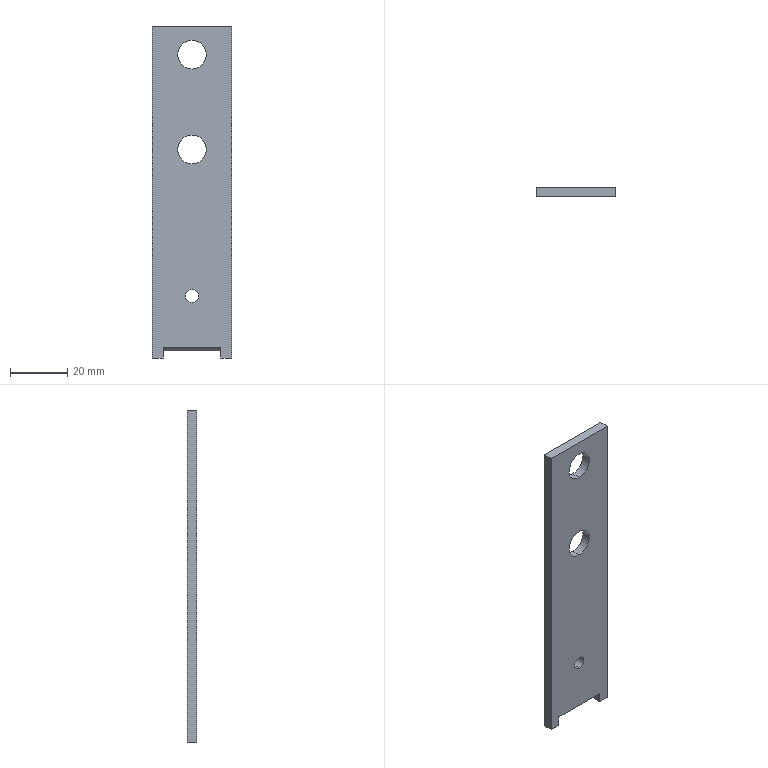Part | SolidWorks | features Chamfer 1, FlatPattern 1, SMBaseFlange 1, SheetMetal 1 | 1 solid | 18 faces | box 27.6 x 3.2 x 115.6 mm | volume 9476 mm3 | plane 12 | cylinder 6 | commonest cylinder face diameters 10 x4 4.5 x2
STEP:
#1=CARTESIAN_POINT('',(13.8,-3.2,-96.25));
#2=VERTEX_POINT('',#1);
#3=CARTESIAN_POINT('',(13.8,-3.2,-91.75));
#4=VERTEX_POINT('',#3);
#5=CARTESIAN_POINT('',(13.8,-3.2,-94.));
#6=DIRECTION('',(0.,1.,0.));
#7=DIRECTION('',(0.,0.,1.));
#8=AXIS2_PLACEMENT_3D('',#5,#6,#7);
#9=CIRCLE('',#8,2.25);
#10=EDGE_CURVE('',#2,#4,#9,.T.);
#11=ORIENTED_EDGE('',*,*,#10,.F.);
#12=CARTESIAN_POINT('',(13.8,0.,-96.25));
#13=VERTEX_POINT('',#12);
#14=CARTESIAN_POINT('',(13.8,-3.2,-96.25));
#15=DIRECTION('',(0.,1.,0.));
#16=VECTOR('',#15,1000.);
#17=LINE('',#14,#16);
#18=EDGE_CURVE('',#2,#13,#17,.T.);
#19=ORIENTED_EDGE('',*,*,#18,.T.);
#20=CARTESIAN_POINT('',(13.8,0.,-91.75));
#21=VERTEX_POINT('',#20);
#22=CARTESIAN_POINT('',(13.8,0.,-94.));
#23=DIRECTION('',(0.,1.,0.));
#24=DIRECTION('',(0.,0.,1.));
#25=AXIS2_PLACEMENT_3D('',#22,#23,#24);
#26=CIRCLE('',#25,2.25);
#27=EDGE_CURVE('',#13,#21,#26,.T.);
#28=ORIENTED_EDGE('',*,*,#27,.T.);
#29=CARTESIAN_POINT('',(13.8,-3.2,-91.75));
#30=DIRECTION('',(0.,1.,0.));
#31=VECTOR('',#30,1000.);
#32=LINE('',#29,#31);
#33=EDGE_CURVE('',#4,#21,#32,.T.);
#34=ORIENTED_EDGE('',*,*,#33,.F.);
#35=EDGE_LOOP('',(#11,#19,#28,#34));
#36=FACE_OUTER_BOUND('',#35,.T.);
#37=CARTESIAN_POINT('',(13.8,-3.2,-94.));
#38=DIRECTION('',(0.,1.,0.));
#39=DIRECTION('',(0.,0.,1.));
#40=AXIS2_PLACEMENT_3D('',#37,#38,#39);
#41=CYLINDRICAL_SURFACE('',#40,2.25);
#42=ADVANCED_FACE('',(#36),#41,.F.);
#43=CARTESIAN_POINT('',(13.8,-3.2,-48.));
#44=VERTEX_POINT('',#43);
#45=CARTESIAN_POINT('',(13.8,-3.2,-38.));
#46=VERTEX_POINT('',#45);
#47=CARTESIAN_POINT('',(13.8,-3.2,-43.));
#48=DIRECTION('',(0.,1.,0.));
#49=DIRECTION('',(0.,0.,1.));
#50=AXIS2_PLACEMENT_3D('',#47,#48,#49);
#51=CIRCLE('',#50,5.);
#52=EDGE_CURVE('',#44,#46,#51,.T.);
#53=ORIENTED_EDGE('',*,*,#52,.F.);
#54=CARTESIAN_POINT('',(13.8,0.,-48.));
#55=VERTEX_POINT('',#54);
#56=CARTESIAN_POINT('',(13.8,-3.2,-48.));
#57=DIRECTION('',(0.,1.,0.));
#58=VECTOR('',#57,1000.);
#59=LINE('',#56,#58);
#60=EDGE_CURVE('',#44,#55,#59,.T.);
#61=ORIENTED_EDGE('',*,*,#60,.T.);
#62=CARTESIAN_POINT('',(13.8,0.,-38.));
#63=VERTEX_POINT('',#62);
#64=CARTESIAN_POINT('',(13.8,0.,-43.));
#65=DIRECTION('',(0.,1.,0.));
#66=DIRECTION('',(0.,0.,1.));
#67=AXIS2_PLACEMENT_3D('',#64,#65,#66);
#68=CIRCLE('',#67,5.);
#69=EDGE_CURVE('',#55,#63,#68,.T.);
#70=ORIENTED_EDGE('',*,*,#69,.T.);
#71=CARTESIAN_POINT('',(13.8,-3.2,-38.));
#72=DIRECTION('',(0.,1.,0.));
#73=VECTOR('',#72,1000.);
#74=LINE('',#71,#73);
#75=EDGE_CURVE('',#46,#63,#74,.T.);
#76=ORIENTED_EDGE('',*,*,#75,.F.);
#77=EDGE_LOOP('',(#53,#61,#70,#76));
#78=FACE_OUTER_BOUND('',#77,.T.);
#79=CARTESIAN_POINT('',(13.8,-3.2,-43.));
#80=DIRECTION('',(0.,1.,0.));
#81=DIRECTION('',(0.,0.,1.));
#82=AXIS2_PLACEMENT_3D('',#79,#80,#81);
#83=CYLINDRICAL_SURFACE('',#82,5.);
#84=ADVANCED_FACE('',(#78),#83,.F.);
#85=CARTESIAN_POINT('',(13.8,-3.2,-15.));
#86=VERTEX_POINT('',#85);
#87=CARTESIAN_POINT('',(13.8,-3.2,-5.));
#88=VERTEX_POINT('',#87);
#89=CARTESIAN_POINT('',(13.8,-3.2,-10.));
#90=DIRECTION('',(0.,1.,0.));
#91=DIRECTION('',(0.,0.,1.));
#92=AXIS2_PLACEMENT_3D('',#89,#90,#91);
#93=CIRCLE('',#92,5.);
#94=EDGE_CURVE('',#86,#88,#93,.T.);
#95=ORIENTED_EDGE('',*,*,#94,.F.);
#96=CARTESIAN_POINT('',(13.8,0.,-15.));
#97=VERTEX_POINT('',#96);
#98=CARTESIAN_POINT('',(13.8,-3.2,-15.));
#99=DIRECTION('',(0.,1.,0.));
#100=VECTOR('',#99,1000.);
#101=LINE('',#98,#100);
#102=EDGE_CURVE('',#86,#97,#101,.T.);
#103=ORIENTED_EDGE('',*,*,#102,.T.);
#104=CARTESIAN_POINT('',(13.8,0.,-5.));
#105=VERTEX_POINT('',#104);
#106=CARTESIAN_POINT('',(13.8,0.,-10.));
#107=DIRECTION('',(0.,1.,0.));
#108=DIRECTION('',(0.,0.,1.));
#109=AXIS2_PLACEMENT_3D('',#106,#107,#108);
#110=CIRCLE('',#109,5.);
#111=EDGE_CURVE('',#97,#105,#110,.T.);
#112=ORIENTED_EDGE('',*,*,#111,.T.);
#113=CARTESIAN_POINT('',(13.8,-3.2,-5.));
#114=DIRECTION('',(0.,1.,0.));
#115=VECTOR('',#114,1000.);
#116=LINE('',#113,#115);
#117=EDGE_CURVE('',#88,#105,#116,.T.);
#118=ORIENTED_EDGE('',*,*,#117,.F.);
#119=EDGE_LOOP('',(#95,#103,#112,#118));
#120=FACE_OUTER_BOUND('',#119,.T.);
#121=CARTESIAN_POINT('',(13.8,-3.2,-10.));
#122=DIRECTION('',(0.,1.,0.));
#123=DIRECTION('',(0.,0.,1.));
#124=AXIS2_PLACEMENT_3D('',#121,#122,#123);
#125=CYLINDRICAL_SURFACE('',#124,5.);
#126=ADVANCED_FACE('',(#120),#125,.F.);
#127=CARTESIAN_POINT('',(0.,0.,-115.6));
#128=VERTEX_POINT('',#127);
#129=CARTESIAN_POINT('',(0.,0.,0.));
#130=VERTEX_POINT('',#129);
#131=CARTESIAN_POINT('',(0.,0.,0.));
#132=DIRECTION('',(0.,0.,1.));
#133=VECTOR('',#132,1000.);
#134=LINE('',#131,#133);
#135=EDGE_CURVE('',#128,#130,#134,.T.);
#136=ORIENTED_EDGE('',*,*,#135,.F.);
#137=CARTESIAN_POINT('',(0.,-3.2,-115.6));
#138=VERTEX_POINT('',#137);
#139=CARTESIAN_POINT('',(0.,-3.2,-115.6));
#140=DIRECTION('',(0.,1.,0.));
#141=VECTOR('',#140,1000.);
#142=LINE('',#139,#141);
#143=EDGE_CURVE('',#138,#128,#142,.T.);
#144=ORIENTED_EDGE('',*,*,#143,.F.);
#145=CARTESIAN_POINT('',(0.,-3.2,0.));
#146=VERTEX_POINT('',#145);
#147=CARTESIAN_POINT('',(0.,-3.2,0.));
#148=DIRECTION('',(0.,0.,1.));
#149=VECTOR('',#148,1000.);
#150=LINE('',#147,#149);
#151=EDGE_CURVE('',#138,#146,#150,.T.);
#152=ORIENTED_EDGE('',*,*,#151,.T.);
#153=CARTESIAN_POINT('',(0.,-3.2,0.));
#154=DIRECTION('',(0.,1.,0.));
#155=VECTOR('',#154,1000.);
#156=LINE('',#153,#155);
#157=EDGE_CURVE('',#146,#130,#156,.T.);
#158=ORIENTED_EDGE('',*,*,#157,.T.);
#159=EDGE_LOOP('',(#136,#144,#152,#158));
#160=FACE_OUTER_BOUND('',#159,.T.);
#161=CARTESIAN_POINT('',(0.,-3.2,0.));
#162=DIRECTION('',(-1.,0.,0.));
#163=DIRECTION('',(0.,0.,1.));
#164=AXIS2_PLACEMENT_3D('',#161,#162,#163);
#165=PLANE('',#164);
#166=ADVANCED_FACE('',(#160),#165,.T.);
#167=CARTESIAN_POINT('',(3.8,0.,-115.6));
#168=VERTEX_POINT('',#167);
#169=CARTESIAN_POINT('',(0.,0.,-115.6));
#170=DIRECTION('',(-1.,0.,0.));
#171=VECTOR('',#170,1000.);
#172=LINE('',#169,#171);
#173=EDGE_CURVE('',#168,#128,#172,.T.);
#174=ORIENTED_EDGE('',*,*,#173,.F.);
#175=CARTESIAN_POINT('',(3.8,-3.2,-115.6));
#176=VERTEX_POINT('',#175);
#177=CARTESIAN_POINT('',(3.8,-3.2,-115.6));
#178=DIRECTION('',(0.,1.,0.));
#179=VECTOR('',#178,1000.);
#180=LINE('',#177,#179);
#181=EDGE_CURVE('',#176,#168,#180,.T.);
#182=ORIENTED_EDGE('',*,*,#181,.F.);
#183=CARTESIAN_POINT('',(0.,-3.2,-115.6));
#184=DIRECTION('',(-1.,0.,0.));
#185=VECTOR('',#184,1000.);
#186=LINE('',#183,#185);
#187=EDGE_CURVE('',#176,#138,#186,.T.);
#188=ORIENTED_EDGE('',*,*,#187,.T.);
#189=ORIENTED_EDGE('',*,*,#143,.T.);
#190=EDGE_LOOP('',(#174,#182,#188,#189));
#191=FACE_OUTER_BOUND('',#190,.T.);
#192=CARTESIAN_POINT('',(0.,-3.2,-115.6));
#193=DIRECTION('',(0.,0.,-1.));
#194=DIRECTION('',(-1.,0.,0.));
#195=AXIS2_PLACEMENT_3D('',#192,#193,#194);
#196=PLANE('',#195);
#197=ADVANCED_FACE('',(#191),#196,.T.);
#198=CARTESIAN_POINT('',(3.8,0.,-112.1));
#199=VERTEX_POINT('',#198);
#200=CARTESIAN_POINT('',(3.8,0.,-115.6));
#201=DIRECTION('',(0.,0.,-1.));
#202=VECTOR('',#201,1000.);
#203=LINE('',#200,#202);
#204=EDGE_CURVE('',#199,#168,#203,.T.);
#205=ORIENTED_EDGE('',*,*,#204,.F.);
#206=CARTESIAN_POINT('',(3.8,-1.,-113.1));
#207=VERTEX_POINT('',#206);
#208=CARTESIAN_POINT('',(3.8,0.,-112.1));
#209=DIRECTION('',(0.,-0.7071,-0.7071));
#210=VECTOR('',#209,1000.);
#211=LINE('',#208,#210);
#212=EDGE_CURVE('',#199,#207,#211,.T.);
#213=ORIENTED_EDGE('',*,*,#212,.T.);
#214=CARTESIAN_POINT('',(3.8,-2.2,-113.1));
#215=VERTEX_POINT('',#214);
#216=CARTESIAN_POINT('',(3.8,-3.2,-113.1));
#217=DIRECTION('',(0.,1.,0.));
#218=VECTOR('',#217,1000.);
#219=LINE('',#216,#218);
#220=EDGE_CURVE('',#215,#207,#219,.T.);
#221=ORIENTED_EDGE('',*,*,#220,.F.);
#222=CARTESIAN_POINT('',(3.8,-3.2,-112.1));
#223=VERTEX_POINT('',#222);
#224=CARTESIAN_POINT('',(3.8,-2.2,-113.1));
#225=DIRECTION('',(0.,-0.7071,0.7071));
#226=VECTOR('',#225,1000.);
#227=LINE('',#224,#226);
#228=EDGE_CURVE('',#215,#223,#227,.T.);
#229=ORIENTED_EDGE('',*,*,#228,.T.);
#230=CARTESIAN_POINT('',(3.8,-3.2,-115.6));
#231=DIRECTION('',(0.,0.,-1.));
#232=VECTOR('',#231,1000.);
#233=LINE('',#230,#232);
#234=EDGE_CURVE('',#223,#176,#233,.T.);
#235=ORIENTED_EDGE('',*,*,#234,.T.);
#236=ORIENTED_EDGE('',*,*,#181,.T.);
#237=EDGE_LOOP('',(#205,#213,#221,#229,#235,#236));
#238=FACE_OUTER_BOUND('',#237,.T.);
#239=CARTESIAN_POINT('',(3.8,-3.2,-115.6));
#240=DIRECTION('',(1.,0.,0.));
#241=DIRECTION('',(0.,0.,-1.));
#242=AXIS2_PLACEMENT_3D('',#239,#240,#241);
#243=PLANE('',#242);
#244=ADVANCED_FACE('',(#238),#243,.T.);
#245=CARTESIAN_POINT('',(23.8,-2.2,-113.1));
#246=VERTEX_POINT('',#245);
#247=CARTESIAN_POINT('',(23.8,-1.,-113.1));
#248=VERTEX_POINT('',#247);
#249=CARTESIAN_POINT('',(23.8,-3.2,-113.1));
#250=DIRECTION('',(0.,1.,0.));
#251=VECTOR('',#250,1000.);
#252=LINE('',#249,#251);
#253=EDGE_CURVE('',#246,#248,#252,.T.);
#254=ORIENTED_EDGE('',*,*,#253,.F.);
#255=CARTESIAN_POINT('',(3.8,-2.2,-113.1));
#256=DIRECTION('',(-1.,0.,0.));
#257=VECTOR('',#256,1000.);
#258=LINE('',#255,#257);
#259=EDGE_CURVE('',#246,#215,#258,.T.);
#260=ORIENTED_EDGE('',*,*,#259,.T.);
#261=ORIENTED_EDGE('',*,*,#220,.T.);
#262=CARTESIAN_POINT('',(23.8,-1.,-113.1));
#263=DIRECTION('',(1.,0.,0.));
#264=VECTOR('',#263,1000.);
#265=LINE('',#262,#264);
#266=EDGE_CURVE('',#207,#248,#265,.T.);
#267=ORIENTED_EDGE('',*,*,#266,.T.);
#268=EDGE_LOOP('',(#254,#260,#261,#267));
#269=FACE_OUTER_BOUND('',#268,.T.);
#270=CARTESIAN_POINT('',(3.8,-3.2,-113.1));
#271=DIRECTION('',(0.,0.,-1.));
#272=DIRECTION('',(-1.,0.,0.));
#273=AXIS2_PLACEMENT_3D('',#270,#271,#272);
#274=PLANE('',#273);
#275=ADVANCED_FACE('',(#269),#274,.T.);
#276=CARTESIAN_POINT('',(23.8,0.,-115.6));
#277=VERTEX_POINT('',#276);
#278=CARTESIAN_POINT('',(23.8,0.,-112.1));
#279=VERTEX_POINT('',#278);
#280=CARTESIAN_POINT('',(23.8,0.,-113.1));
#281=DIRECTION('',(0.,0.,1.));
#282=VECTOR('',#281,1000.);
#283=LINE('',#280,#282);
#284=EDGE_CURVE('',#277,#279,#283,.T.);
#285=ORIENTED_EDGE('',*,*,#284,.F.);
#286=CARTESIAN_POINT('',(23.8,-3.2,-115.6));
#287=VERTEX_POINT('',#286);
#288=CARTESIAN_POINT('',(23.8,-3.2,-115.6));
#289=DIRECTION('',(0.,1.,0.));
#290=VECTOR('',#289,1000.);
#291=LINE('',#288,#290);
#292=EDGE_CURVE('',#287,#277,#291,.T.);
#293=ORIENTED_EDGE('',*,*,#292,.F.);
#294=CARTESIAN_POINT('',(23.8,-3.2,-112.1));
#295=VERTEX_POINT('',#294);
#296=CARTESIAN_POINT('',(23.8,-3.2,-113.1));
#297=DIRECTION('',(0.,0.,1.));
#298=VECTOR('',#297,1000.);
#299=LINE('',#296,#298);
#300=EDGE_CURVE('',#287,#295,#299,.T.);
#301=ORIENTED_EDGE('',*,*,#300,.T.);
#302=CARTESIAN_POINT('',(23.8,-2.2,-113.1));
#303=DIRECTION('',(0.,0.7071,-0.7071));
#304=VECTOR('',#303,1000.);
#305=LINE('',#302,#304);
#306=EDGE_CURVE('',#295,#246,#305,.T.);
#307=ORIENTED_EDGE('',*,*,#306,.T.);
#308=ORIENTED_EDGE('',*,*,#253,.T.);
#309=CARTESIAN_POINT('',(23.8,0.,-112.1));
#310=DIRECTION('',(0.,0.7071,0.7071));
#311=VECTOR('',#310,1000.);
#312=LINE('',#309,#311);
#313=EDGE_CURVE('',#248,#279,#312,.T.);
#314=ORIENTED_EDGE('',*,*,#313,.T.);
#315=EDGE_LOOP('',(#285,#293,#301,#307,#308,#314));
#316=FACE_OUTER_BOUND('',#315,.T.);
#317=CARTESIAN_POINT('',(23.8,-3.2,-113.1));
#318=DIRECTION('',(-1.,0.,0.));
#319=DIRECTION('',(0.,0.,1.));
#320=AXIS2_PLACEMENT_3D('',#317,#318,#319);
#321=PLANE('',#320);
#322=ADVANCED_FACE('',(#316),#321,.T.);
#323=CARTESIAN_POINT('',(27.6,0.,-115.6));
#324=VERTEX_POINT('',#323);
#325=CARTESIAN_POINT('',(23.8,0.,-115.6));
#326=DIRECTION('',(-1.,0.,0.));
#327=VECTOR('',#326,1000.);
#328=LINE('',#325,#327);
#329=EDGE_CURVE('',#324,#277,#328,.T.);
#330=ORIENTED_EDGE('',*,*,#329,.F.);
#331=CARTESIAN_POINT('',(27.6,-3.2,-115.6));
#332=VERTEX_POINT('',#331);
#333=CARTESIAN_POINT('',(27.6,-3.2,-115.6));
#334=DIRECTION('',(0.,1.,0.));
#335=VECTOR('',#334,1000.);
#336=LINE('',#333,#335);
#337=EDGE_CURVE('',#332,#324,#336,.T.);
#338=ORIENTED_EDGE('',*,*,#337,.F.);
#339=CARTESIAN_POINT('',(23.8,-3.2,-115.6));
#340=DIRECTION('',(-1.,0.,0.));
#341=VECTOR('',#340,1000.);
#342=LINE('',#339,#341);
#343=EDGE_CURVE('',#332,#287,#342,.T.);
#344=ORIENTED_EDGE('',*,*,#343,.T.);
#345=ORIENTED_EDGE('',*,*,#292,.T.);
#346=EDGE_LOOP('',(#330,#338,#344,#345));
#347=FACE_OUTER_BOUND('',#346,.T.);
#348=CARTESIAN_POINT('',(23.8,-3.2,-115.6));
#349=DIRECTION('',(0.,0.,-1.));
#350=DIRECTION('',(-1.,0.,0.));
#351=AXIS2_PLACEMENT_3D('',#348,#349,#350);
#352=PLANE('',#351);
#353=ADVANCED_FACE('',(#347),#352,.T.);
#354=CARTESIAN_POINT('',(27.6,0.,0.));
#355=VERTEX_POINT('',#354);
#356=CARTESIAN_POINT('',(27.6,0.,0.));
#357=DIRECTION('',(0.,0.,-1.));
#358=VECTOR('',#357,1000.);
#359=LINE('',#356,#358);
#360=EDGE_CURVE('',#355,#324,#359,.T.);
#361=ORIENTED_EDGE('',*,*,#360,.F.);
#362=CARTESIAN_POINT('',(27.6,-3.2,0.));
#363=VERTEX_POINT('',#362);
#364=CARTESIAN_POINT('',(27.6,-3.2,0.));
#365=DIRECTION('',(0.,1.,0.));
#366=VECTOR('',#365,1000.);
#367=LINE('',#364,#366);
#368=EDGE_CURVE('',#363,#355,#367,.T.);
#369=ORIENTED_EDGE('',*,*,#368,.F.);
#370=CARTESIAN_POINT('',(27.6,-3.2,0.));
#371=DIRECTION('',(0.,0.,-1.));
#372=VECTOR('',#371,1000.);
#373=LINE('',#370,#372);
#374=EDGE_CURVE('',#363,#332,#373,.T.);
#375=ORIENTED_EDGE('',*,*,#374,.T.);
#376=ORIENTED_EDGE('',*,*,#337,.T.);
#377=EDGE_LOOP('',(#361,#369,#375,#376));
#378=FACE_OUTER_BOUND('',#377,.T.);
#379=CARTESIAN_POINT('',(27.6,-3.2,0.));
#380=DIRECTION('',(1.,0.,0.));
#381=DIRECTION('',(0.,0.,-1.));
#382=AXIS2_PLACEMENT_3D('',#379,#380,#381);
#383=PLANE('',#382);
#384=ADVANCED_FACE('',(#378),#383,.T.);
#385=CARTESIAN_POINT('',(0.,0.,0.));
#386=DIRECTION('',(1.,0.,0.));
#387=VECTOR('',#386,1000.);
#388=LINE('',#385,#387);
#389=EDGE_CURVE('',#130,#355,#388,.T.);
#390=ORIENTED_EDGE('',*,*,#389,.F.);
#391=ORIENTED_EDGE('',*,*,#157,.F.);
#392=CARTESIAN_POINT('',(0.,-3.2,0.));
#393=DIRECTION('',(1.,0.,0.));
#394=VECTOR('',#393,1000.);
#395=LINE('',#392,#394);
#396=EDGE_CURVE('',#146,#363,#395,.T.);
#397=ORIENTED_EDGE('',*,*,#396,.T.);
#398=ORIENTED_EDGE('',*,*,#368,.T.);
#399=EDGE_LOOP('',(#390,#391,#397,#398));
#400=FACE_OUTER_BOUND('',#399,.T.);
#401=CARTESIAN_POINT('',(0.,-3.2,0.));
#402=DIRECTION('',(0.,0.,1.));
#403=DIRECTION('',(1.,0.,0.));
#404=AXIS2_PLACEMENT_3D('',#401,#402,#403);
#405=PLANE('',#404);
#406=ADVANCED_FACE('',(#400),#405,.T.);
#407=CARTESIAN_POINT('',(13.8,-3.2,-94.));
#408=DIRECTION('',(0.,1.,0.));
#409=DIRECTION('',(0.,0.,1.));
#410=AXIS2_PLACEMENT_3D('',#407,#408,#409);
#411=CIRCLE('',#410,2.25);
#412=EDGE_CURVE('',#4,#2,#411,.T.);
#413=ORIENTED_EDGE('',*,*,#412,.T.);
#414=ORIENTED_EDGE('',*,*,#10,.T.);
#415=EDGE_LOOP('',(#413,#414));
#416=FACE_BOUND('',#415,.T.);
#417=CARTESIAN_POINT('',(13.8,-3.2,-43.));
#418=DIRECTION('',(0.,1.,0.));
#419=DIRECTION('',(0.,0.,1.));
#420=AXIS2_PLACEMENT_3D('',#417,#418,#419);
#421=CIRCLE('',#420,5.);
#422=EDGE_CURVE('',#46,#44,#421,.T.);
#423=ORIENTED_EDGE('',*,*,#422,.T.);
#424=ORIENTED_EDGE('',*,*,#52,.T.);
#425=EDGE_LOOP('',(#423,#424));
#426=FACE_BOUND('',#425,.T.);
#427=CARTESIAN_POINT('',(13.8,-3.2,-10.));
#428=DIRECTION('',(0.,1.,0.));
#429=DIRECTION('',(0.,0.,1.));
#430=AXIS2_PLACEMENT_3D('',#427,#428,#429);
#431=CIRCLE('',#430,5.);
#432=EDGE_CURVE('',#88,#86,#431,.T.);
#433=ORIENTED_EDGE('',*,*,#432,.T.);
#434=ORIENTED_EDGE('',*,*,#94,.T.);
#435=EDGE_LOOP('',(#433,#434));
#436=FACE_BOUND('',#435,.T.);
#437=ORIENTED_EDGE('',*,*,#234,.F.);
#438=CARTESIAN_POINT('',(0.,-3.2,-112.1));
#439=DIRECTION('',(1.,0.,0.));
#440=VECTOR('',#439,1000.);
#441=LINE('',#438,#440);
#442=EDGE_CURVE('',#223,#295,#441,.T.);
#443=ORIENTED_EDGE('',*,*,#442,.T.);
#444=ORIENTED_EDGE('',*,*,#300,.F.);
#445=ORIENTED_EDGE('',*,*,#343,.F.);
#446=ORIENTED_EDGE('',*,*,#374,.F.);
#447=ORIENTED_EDGE('',*,*,#396,.F.);
#448=ORIENTED_EDGE('',*,*,#151,.F.);
#449=ORIENTED_EDGE('',*,*,#187,.F.);
#450=EDGE_LOOP('',(#437,#443,#444,#445,#446,#447,#448,#449));
#451=FACE_OUTER_BOUND('',#450,.T.);
#452=CARTESIAN_POINT('',(0.,-3.2,0.));
#453=DIRECTION('',(0.,-1.,0.));
#454=DIRECTION('',(0.,0.,-1.));
#455=AXIS2_PLACEMENT_3D('',#452,#453,#454);
#456=PLANE('',#455);
#457=ADVANCED_FACE('',(#416,#426,#436,#451),#456,.T.);
#458=CARTESIAN_POINT('',(13.8,0.,-94.));
#459=DIRECTION('',(0.,1.,0.));
#460=DIRECTION('',(0.,0.,1.));
#461=AXIS2_PLACEMENT_3D('',#458,#459,#460);
#462=CIRCLE('',#461,2.25);
#463=EDGE_CURVE('',#21,#13,#462,.T.);
#464=ORIENTED_EDGE('',*,*,#463,.F.);
#465=ORIENTED_EDGE('',*,*,#27,.F.);
#466=EDGE_LOOP('',(#464,#465));
#467=FACE_BOUND('',#466,.T.);
#468=CARTESIAN_POINT('',(13.8,0.,-43.));
#469=DIRECTION('',(0.,1.,0.));
#470=DIRECTION('',(0.,0.,1.));
#471=AXIS2_PLACEMENT_3D('',#468,#469,#470);
#472=CIRCLE('',#471,5.);
#473=EDGE_CURVE('',#63,#55,#472,.T.);
#474=ORIENTED_EDGE('',*,*,#473,.F.);
#475=ORIENTED_EDGE('',*,*,#69,.F.);
#476=EDGE_LOOP('',(#474,#475));
#477=FACE_BOUND('',#476,.T.);
#478=CARTESIAN_POINT('',(13.8,0.,-10.));
#479=DIRECTION('',(0.,1.,0.));
#480=DIRECTION('',(0.,0.,1.));
#481=AXIS2_PLACEMENT_3D('',#478,#479,#480);
#482=CIRCLE('',#481,5.);
#483=EDGE_CURVE('',#105,#97,#482,.T.);
#484=ORIENTED_EDGE('',*,*,#483,.F.);
#485=ORIENTED_EDGE('',*,*,#111,.F.);
#486=EDGE_LOOP('',(#484,#485));
#487=FACE_BOUND('',#486,.T.);
#488=CARTESIAN_POINT('',(3.8,0.,-112.1));
#489=DIRECTION('',(-1.,0.,0.));
#490=VECTOR('',#489,1000.);
#491=LINE('',#488,#490);
#492=EDGE_CURVE('',#279,#199,#491,.T.);
#493=ORIENTED_EDGE('',*,*,#492,.T.);
#494=ORIENTED_EDGE('',*,*,#204,.T.);
#495=ORIENTED_EDGE('',*,*,#173,.T.);
#496=ORIENTED_EDGE('',*,*,#135,.T.);
#497=ORIENTED_EDGE('',*,*,#389,.T.);
#498=ORIENTED_EDGE('',*,*,#360,.T.);
#499=ORIENTED_EDGE('',*,*,#329,.T.);
#500=ORIENTED_EDGE('',*,*,#284,.T.);
#501=EDGE_LOOP('',(#493,#494,#495,#496,#497,#498,#499,#500));
#502=FACE_OUTER_BOUND('',#501,.T.);
#503=CARTESIAN_POINT('',(0.,0.,0.));
#504=DIRECTION('',(0.,-1.,0.));
#505=DIRECTION('',(0.,0.,-1.));
#506=AXIS2_PLACEMENT_3D('',#503,#504,#505);
#507=PLANE('',#506);
#508=ADVANCED_FACE('',(#467,#477,#487,#502),#507,.F.);
#509=ORIENTED_EDGE('',*,*,#102,.F.);
#510=ORIENTED_EDGE('',*,*,#432,.F.);
#511=ORIENTED_EDGE('',*,*,#117,.T.);
#512=ORIENTED_EDGE('',*,*,#483,.T.);
#513=EDGE_LOOP('',(#509,#510,#511,#512));
#514=FACE_OUTER_BOUND('',#513,.T.);
#515=CARTESIAN_POINT('',(13.8,-3.2,-10.));
#516=DIRECTION('',(0.,1.,0.));
#517=DIRECTION('',(0.,0.,1.));
#518=AXIS2_PLACEMENT_3D('',#515,#516,#517);
#519=CYLINDRICAL_SURFACE('',#518,5.);
#520=ADVANCED_FACE('',(#514),#519,.F.);
#521=ORIENTED_EDGE('',*,*,#60,.F.);
#522=ORIENTED_EDGE('',*,*,#422,.F.);
#523=ORIENTED_EDGE('',*,*,#75,.T.);
#524=ORIENTED_EDGE('',*,*,#473,.T.);
#525=EDGE_LOOP('',(#521,#522,#523,#524));
#526=FACE_OUTER_BOUND('',#525,.T.);
#527=CARTESIAN_POINT('',(13.8,-3.2,-43.));
#528=DIRECTION('',(0.,1.,0.));
#529=DIRECTION('',(0.,0.,1.));
#530=AXIS2_PLACEMENT_3D('',#527,#528,#529);
#531=CYLINDRICAL_SURFACE('',#530,5.);
#532=ADVANCED_FACE('',(#526),#531,.F.);
#533=ORIENTED_EDGE('',*,*,#18,.F.);
#534=ORIENTED_EDGE('',*,*,#412,.F.);
#535=ORIENTED_EDGE('',*,*,#33,.T.);
#536=ORIENTED_EDGE('',*,*,#463,.T.);
#537=EDGE_LOOP('',(#533,#534,#535,#536));
#538=FACE_OUTER_BOUND('',#537,.T.);
#539=CARTESIAN_POINT('',(13.8,-3.2,-94.));
#540=DIRECTION('',(0.,1.,0.));
#541=DIRECTION('',(0.,0.,1.));
#542=AXIS2_PLACEMENT_3D('',#539,#540,#541);
#543=CYLINDRICAL_SURFACE('',#542,2.25);
#544=ADVANCED_FACE('',(#538),#543,.F.);
#545=ORIENTED_EDGE('',*,*,#306,.F.);
#546=ORIENTED_EDGE('',*,*,#442,.F.);
#547=ORIENTED_EDGE('',*,*,#228,.F.);
#548=ORIENTED_EDGE('',*,*,#259,.F.);
#549=EDGE_LOOP('',(#545,#546,#547,#548));
#550=FACE_OUTER_BOUND('',#549,.T.);
#551=CARTESIAN_POINT('',(3.8,-2.2,-113.1));
#552=DIRECTION('',(0.,0.7071,0.7071));
#553=DIRECTION('',(-1.,0.,0.));
#554=AXIS2_PLACEMENT_3D('',#551,#552,#553);
#555=PLANE('',#554);
#556=ADVANCED_FACE('',(#550),#555,.F.);
#557=ORIENTED_EDGE('',*,*,#313,.F.);
#558=ORIENTED_EDGE('',*,*,#266,.F.);
#559=ORIENTED_EDGE('',*,*,#212,.F.);
#560=ORIENTED_EDGE('',*,*,#492,.F.);
#561=EDGE_LOOP('',(#557,#558,#559,#560));
#562=FACE_OUTER_BOUND('',#561,.T.);
#563=CARTESIAN_POINT('',(0.,0.,-112.1));
#564=DIRECTION('',(0.,0.7071,-0.7071));
#565=DIRECTION('',(1.,0.,0.));
#566=AXIS2_PLACEMENT_3D('',#563,#564,#565);
#567=PLANE('',#566);
#568=ADVANCED_FACE('',(#562),#567,.T.);
#569=CLOSED_SHELL('',(#42,#84,#126,#166,#197,#244,#275,#322,#353,#384,#406,#457,#508,#520,#532,#544,#556,#568));
#570=MANIFOLD_SOLID_BREP('',#569);
#571=CARTESIAN_POINT('',(0.,0.,0.));
#572=DIRECTION('',(0.,0.,1.));
#573=DIRECTION('',(1.,0.,0.));
#574=AXIS2_PLACEMENT_3D('',#571,#572,#573);
#575=(LENGTH_UNIT()NAMED_UNIT(*)SI_UNIT(.MILLI.,.METRE.));
#576=UNCERTAINTY_MEASURE_WITH_UNIT(LENGTH_MEASURE(0.00001),#575,'','');
#577=(NAMED_UNIT(*)PLANE_ANGLE_UNIT()SI_UNIT($,.RADIAN.));
#578=(NAMED_UNIT(*)SI_UNIT($,.STERADIAN.)SOLID_ANGLE_UNIT());
#579=(GEOMETRIC_REPRESENTATION_CONTEXT(3)GLOBAL_UNCERTAINTY_ASSIGNED_CONTEXT((#576))GLOBAL_UNIT_ASSIGNED_CONTEXT((#575,#577,#578))REPRESENTATION_CONTEXT('',''));
#580=ADVANCED_BREP_SHAPE_REPRESENTATION('',(#570,#574),#579);